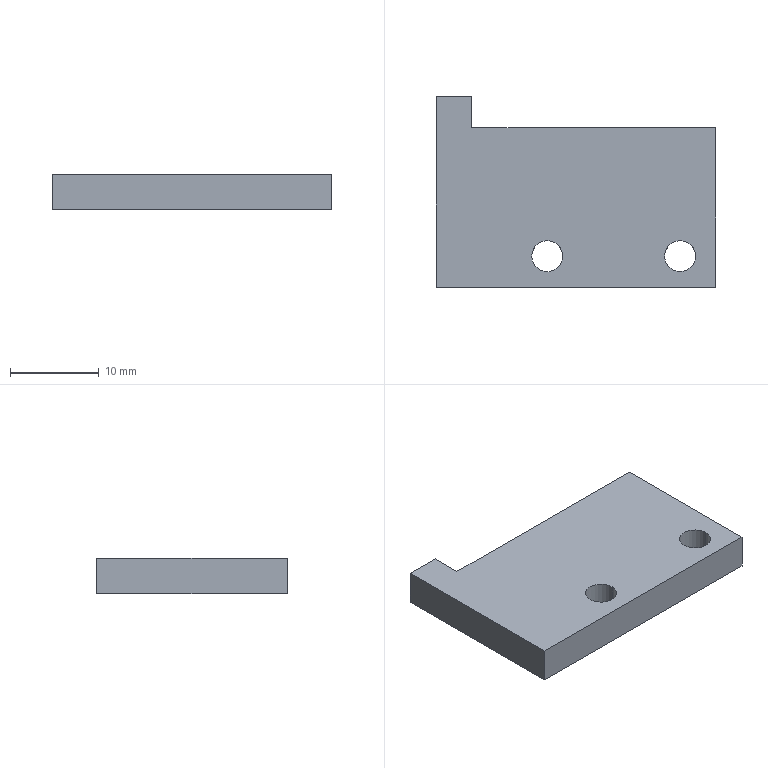Part | NX | 1 solid | 12 faces | box 31.5 x 21.5 x 4 mm | volume 2247 mm3 | plane 8 | cylinder 4 | commonest cylinder face diameters 3.5 x4
STEP:
#1=CARTESIAN_POINT('',(0.,-21.5,0.));
#2=VERTEX_POINT('',#1);
#3=CARTESIAN_POINT('',(0.,0.,0.));
#4=VERTEX_POINT('',#3);
#5=CARTESIAN_POINT('',(0.,0.,0.));
#6=DIRECTION('',(0.,1.,0.));
#7=VECTOR('',#6,1000.);
#8=LINE('',#5,#7);
#9=EDGE_CURVE('',#2,#4,#8,.T.);
#10=ORIENTED_EDGE('',*,*,#9,.T.);
#11=CARTESIAN_POINT('',(4.,0.,0.));
#12=VERTEX_POINT('',#11);
#13=CARTESIAN_POINT('',(0.,0.,0.));
#14=DIRECTION('',(1.,0.,0.));
#15=VECTOR('',#14,1000.);
#16=LINE('',#13,#15);
#17=EDGE_CURVE('',#4,#12,#16,.T.);
#18=ORIENTED_EDGE('',*,*,#17,.T.);
#19=CARTESIAN_POINT('',(4.,-3.5,0.));
#20=VERTEX_POINT('',#19);
#21=CARTESIAN_POINT('',(4.,0.,0.));
#22=DIRECTION('',(0.,-1.,0.));
#23=VECTOR('',#22,1000.);
#24=LINE('',#21,#23);
#25=EDGE_CURVE('',#12,#20,#24,.T.);
#26=ORIENTED_EDGE('',*,*,#25,.T.);
#27=CARTESIAN_POINT('',(31.5,-3.5,0.));
#28=VERTEX_POINT('',#27);
#29=CARTESIAN_POINT('',(0.,-3.5,0.));
#30=DIRECTION('',(1.,0.,0.));
#31=VECTOR('',#30,1000.);
#32=LINE('',#29,#31);
#33=EDGE_CURVE('',#20,#28,#32,.T.);
#34=ORIENTED_EDGE('',*,*,#33,.T.);
#35=CARTESIAN_POINT('',(31.5,-21.5,0.));
#36=VERTEX_POINT('',#35);
#37=CARTESIAN_POINT('',(31.5,0.,0.));
#38=DIRECTION('',(0.,1.,0.));
#39=VECTOR('',#38,1000.);
#40=LINE('',#37,#39);
#41=EDGE_CURVE('',#36,#28,#40,.T.);
#42=ORIENTED_EDGE('',*,*,#41,.F.);
#43=CARTESIAN_POINT('',(0.,-21.5,0.));
#44=DIRECTION('',(-1.,0.,0.));
#45=VECTOR('',#44,1000.);
#46=LINE('',#43,#45);
#47=EDGE_CURVE('',#36,#2,#46,.T.);
#48=ORIENTED_EDGE('',*,*,#47,.T.);
#49=EDGE_LOOP('',(#10,#18,#26,#34,#42,#48));
#50=FACE_BOUND('',#49,.T.);
#51=CARTESIAN_POINT('',(29.25,-18.,0.));
#52=VERTEX_POINT('',#51);
#53=CARTESIAN_POINT('',(25.75,-18.,0.));
#54=VERTEX_POINT('',#53);
#55=CARTESIAN_POINT('',(27.5,-18.,0.));
#56=DIRECTION('',(0.,0.,-1.));
#57=DIRECTION('',(-1.,0.,0.));
#58=AXIS2_PLACEMENT_3D('',#55,#56,#57);
#59=CIRCLE('',#58,1.75);
#60=EDGE_CURVE('',#52,#54,#59,.T.);
#61=ORIENTED_EDGE('',*,*,#60,.F.);
#62=CARTESIAN_POINT('',(27.5,-18.,0.));
#63=DIRECTION('',(0.,0.,-1.));
#64=DIRECTION('',(-1.,0.,0.));
#65=AXIS2_PLACEMENT_3D('',#62,#63,#64);
#66=CIRCLE('',#65,1.75);
#67=EDGE_CURVE('',#54,#52,#66,.T.);
#68=ORIENTED_EDGE('',*,*,#67,.F.);
#69=EDGE_LOOP('',(#61,#68));
#70=FACE_BOUND('',#69,.T.);
#71=CARTESIAN_POINT('',(14.25,-18.,0.));
#72=VERTEX_POINT('',#71);
#73=CARTESIAN_POINT('',(10.75,-18.,0.));
#74=VERTEX_POINT('',#73);
#75=CARTESIAN_POINT('',(12.5,-18.,0.));
#76=DIRECTION('',(0.,0.,-1.));
#77=DIRECTION('',(-1.,0.,0.));
#78=AXIS2_PLACEMENT_3D('',#75,#76,#77);
#79=CIRCLE('',#78,1.75);
#80=EDGE_CURVE('',#72,#74,#79,.T.);
#81=ORIENTED_EDGE('',*,*,#80,.F.);
#82=CARTESIAN_POINT('',(12.5,-18.,0.));
#83=DIRECTION('',(0.,0.,-1.));
#84=DIRECTION('',(-1.,0.,0.));
#85=AXIS2_PLACEMENT_3D('',#82,#83,#84);
#86=CIRCLE('',#85,1.75);
#87=EDGE_CURVE('',#74,#72,#86,.T.);
#88=ORIENTED_EDGE('',*,*,#87,.F.);
#89=EDGE_LOOP('',(#81,#88));
#90=FACE_BOUND('',#89,.T.);
#91=CARTESIAN_POINT('',(0.,0.,0.));
#92=DIRECTION('',(0.,0.,1.));
#93=DIRECTION('',(1.,0.,0.));
#94=AXIS2_PLACEMENT_3D('',#91,#92,#93);
#95=PLANE('',#94);
#96=ADVANCED_FACE('',(#50,#70,#90),#95,.F.);
#97=CARTESIAN_POINT('',(4.,0.,4.));
#98=VERTEX_POINT('',#97);
#99=CARTESIAN_POINT('',(4.,0.,0.));
#100=DIRECTION('',(0.,0.,1.));
#101=VECTOR('',#100,1000.);
#102=LINE('',#99,#101);
#103=EDGE_CURVE('',#12,#98,#102,.T.);
#104=ORIENTED_EDGE('',*,*,#103,.T.);
#105=CARTESIAN_POINT('',(4.,-3.5,4.));
#106=VERTEX_POINT('',#105);
#107=CARTESIAN_POINT('',(4.,0.,4.));
#108=DIRECTION('',(0.,1.,0.));
#109=VECTOR('',#108,1000.);
#110=LINE('',#107,#109);
#111=EDGE_CURVE('',#106,#98,#110,.T.);
#112=ORIENTED_EDGE('',*,*,#111,.F.);
#113=CARTESIAN_POINT('',(4.,-3.5,0.));
#114=DIRECTION('',(0.,0.,-1.));
#115=VECTOR('',#114,1000.);
#116=LINE('',#113,#115);
#117=EDGE_CURVE('',#106,#20,#116,.T.);
#118=ORIENTED_EDGE('',*,*,#117,.T.);
#119=ORIENTED_EDGE('',*,*,#25,.F.);
#120=EDGE_LOOP('',(#104,#112,#118,#119));
#121=FACE_BOUND('',#120,.T.);
#122=CARTESIAN_POINT('',(4.,0.,5.));
#123=DIRECTION('',(-1.,0.,0.));
#124=DIRECTION('',(0.,0.,1.));
#125=AXIS2_PLACEMENT_3D('',#122,#123,#124);
#126=PLANE('',#125);
#127=ADVANCED_FACE('',(#121),#126,.F.);
#128=CARTESIAN_POINT('',(0.,0.,4.));
#129=VERTEX_POINT('',#128);
#130=CARTESIAN_POINT('',(0.,0.,0.));
#131=DIRECTION('',(0.,0.,-1.));
#132=VECTOR('',#131,1000.);
#133=LINE('',#130,#132);
#134=EDGE_CURVE('',#129,#4,#133,.T.);
#135=ORIENTED_EDGE('',*,*,#134,.F.);
#136=CARTESIAN_POINT('',(0.,0.,4.));
#137=DIRECTION('',(-1.,0.,0.));
#138=VECTOR('',#137,1000.);
#139=LINE('',#136,#138);
#140=EDGE_CURVE('',#98,#129,#139,.T.);
#141=ORIENTED_EDGE('',*,*,#140,.F.);
#142=ORIENTED_EDGE('',*,*,#103,.F.);
#143=ORIENTED_EDGE('',*,*,#17,.F.);
#144=EDGE_LOOP('',(#135,#141,#142,#143));
#145=FACE_BOUND('',#144,.T.);
#146=CARTESIAN_POINT('',(32.,0.,0.));
#147=DIRECTION('',(0.,1.,0.));
#148=DIRECTION('',(1.,0.,0.));
#149=AXIS2_PLACEMENT_3D('',#146,#147,#148);
#150=PLANE('',#149);
#151=ADVANCED_FACE('',(#145),#150,.T.);
#152=CARTESIAN_POINT('',(0.,-21.5,4.));
#153=VERTEX_POINT('',#152);
#154=CARTESIAN_POINT('',(0.,-21.5,0.));
#155=DIRECTION('',(0.,0.,1.));
#156=VECTOR('',#155,1000.);
#157=LINE('',#154,#156);
#158=EDGE_CURVE('',#2,#153,#157,.T.);
#159=ORIENTED_EDGE('',*,*,#158,.T.);
#160=CARTESIAN_POINT('',(0.,0.,4.));
#161=DIRECTION('',(0.,-1.,0.));
#162=VECTOR('',#161,1000.);
#163=LINE('',#160,#162);
#164=EDGE_CURVE('',#129,#153,#163,.T.);
#165=ORIENTED_EDGE('',*,*,#164,.F.);
#166=ORIENTED_EDGE('',*,*,#134,.T.);
#167=ORIENTED_EDGE('',*,*,#9,.F.);
#168=EDGE_LOOP('',(#159,#165,#166,#167));
#169=FACE_BOUND('',#168,.T.);
#170=CARTESIAN_POINT('',(0.,0.,0.));
#171=DIRECTION('',(-1.,0.,0.));
#172=DIRECTION('',(0.,0.,1.));
#173=AXIS2_PLACEMENT_3D('',#170,#171,#172);
#174=PLANE('',#173);
#175=ADVANCED_FACE('',(#169),#174,.T.);
#176=CARTESIAN_POINT('',(31.5,-21.5,4.));
#177=VERTEX_POINT('',#176);
#178=CARTESIAN_POINT('',(0.,-21.5,4.));
#179=DIRECTION('',(1.,0.,0.));
#180=VECTOR('',#179,1000.);
#181=LINE('',#178,#180);
#182=EDGE_CURVE('',#153,#177,#181,.T.);
#183=ORIENTED_EDGE('',*,*,#182,.T.);
#184=CARTESIAN_POINT('',(31.5,-3.5,4.));
#185=VERTEX_POINT('',#184);
#186=CARTESIAN_POINT('',(31.5,0.,4.));
#187=DIRECTION('',(0.,-1.,0.));
#188=VECTOR('',#187,1000.);
#189=LINE('',#186,#188);
#190=EDGE_CURVE('',#185,#177,#189,.T.);
#191=ORIENTED_EDGE('',*,*,#190,.F.);
#192=CARTESIAN_POINT('',(0.,-3.5,4.));
#193=DIRECTION('',(1.,0.,0.));
#194=VECTOR('',#193,1000.);
#195=LINE('',#192,#194);
#196=EDGE_CURVE('',#106,#185,#195,.T.);
#197=ORIENTED_EDGE('',*,*,#196,.F.);
#198=ORIENTED_EDGE('',*,*,#111,.T.);
#199=ORIENTED_EDGE('',*,*,#140,.T.);
#200=ORIENTED_EDGE('',*,*,#164,.T.);
#201=EDGE_LOOP('',(#183,#191,#197,#198,#199,#200));
#202=FACE_BOUND('',#201,.T.);
#203=CARTESIAN_POINT('',(29.25,-18.,4.));
#204=VERTEX_POINT('',#203);
#205=CARTESIAN_POINT('',(25.75,-18.,4.));
#206=VERTEX_POINT('',#205);
#207=CARTESIAN_POINT('',(27.5,-18.,4.));
#208=DIRECTION('',(0.,0.,-1.));
#209=DIRECTION('',(-1.,0.,0.));
#210=AXIS2_PLACEMENT_3D('',#207,#208,#209);
#211=CIRCLE('',#210,1.75);
#212=EDGE_CURVE('',#204,#206,#211,.T.);
#213=ORIENTED_EDGE('',*,*,#212,.T.);
#214=CARTESIAN_POINT('',(27.5,-18.,4.));
#215=DIRECTION('',(0.,0.,-1.));
#216=DIRECTION('',(-1.,0.,0.));
#217=AXIS2_PLACEMENT_3D('',#214,#215,#216);
#218=CIRCLE('',#217,1.75);
#219=EDGE_CURVE('',#206,#204,#218,.T.);
#220=ORIENTED_EDGE('',*,*,#219,.T.);
#221=EDGE_LOOP('',(#213,#220));
#222=FACE_BOUND('',#221,.T.);
#223=CARTESIAN_POINT('',(10.75,-18.,4.));
#224=VERTEX_POINT('',#223);
#225=CARTESIAN_POINT('',(14.25,-18.,4.));
#226=VERTEX_POINT('',#225);
#227=CARTESIAN_POINT('',(12.5,-18.,4.));
#228=DIRECTION('',(0.,0.,-1.));
#229=DIRECTION('',(-1.,0.,0.));
#230=AXIS2_PLACEMENT_3D('',#227,#228,#229);
#231=CIRCLE('',#230,1.75);
#232=EDGE_CURVE('',#224,#226,#231,.T.);
#233=ORIENTED_EDGE('',*,*,#232,.T.);
#234=CARTESIAN_POINT('',(12.5,-18.,4.));
#235=DIRECTION('',(0.,0.,-1.));
#236=DIRECTION('',(-1.,0.,0.));
#237=AXIS2_PLACEMENT_3D('',#234,#235,#236);
#238=CIRCLE('',#237,1.75);
#239=EDGE_CURVE('',#226,#224,#238,.T.);
#240=ORIENTED_EDGE('',*,*,#239,.T.);
#241=EDGE_LOOP('',(#233,#240));
#242=FACE_BOUND('',#241,.T.);
#243=CARTESIAN_POINT('',(32.,-21.5,4.));
#244=DIRECTION('',(0.,0.,-1.));
#245=DIRECTION('',(0.,-1.,0.));
#246=AXIS2_PLACEMENT_3D('',#243,#244,#245);
#247=PLANE('',#246);
#248=ADVANCED_FACE('',(#202,#222,#242),#247,.F.);
#249=CARTESIAN_POINT('',(31.5,-3.5,0.));
#250=DIRECTION('',(0.,0.,1.));
#251=VECTOR('',#250,1000.);
#252=LINE('',#249,#251);
#253=EDGE_CURVE('',#28,#185,#252,.T.);
#254=ORIENTED_EDGE('',*,*,#253,.F.);
#255=ORIENTED_EDGE('',*,*,#33,.F.);
#256=ORIENTED_EDGE('',*,*,#117,.F.);
#257=ORIENTED_EDGE('',*,*,#196,.T.);
#258=EDGE_LOOP('',(#254,#255,#256,#257));
#259=FACE_BOUND('',#258,.T.);
#260=CARTESIAN_POINT('',(3.,-3.5,5.));
#261=DIRECTION('',(0.,-1.,0.));
#262=DIRECTION('',(0.,0.,-1.));
#263=AXIS2_PLACEMENT_3D('',#260,#261,#262);
#264=PLANE('',#263);
#265=ADVANCED_FACE('',(#259),#264,.F.);
#266=ORIENTED_EDGE('',*,*,#253,.T.);
#267=ORIENTED_EDGE('',*,*,#190,.T.);
#268=CARTESIAN_POINT('',(31.5,-21.5,0.));
#269=DIRECTION('',(0.,0.,1.));
#270=VECTOR('',#269,1000.);
#271=LINE('',#268,#270);
#272=EDGE_CURVE('',#36,#177,#271,.T.);
#273=ORIENTED_EDGE('',*,*,#272,.F.);
#274=ORIENTED_EDGE('',*,*,#41,.T.);
#275=EDGE_LOOP('',(#266,#267,#273,#274));
#276=FACE_BOUND('',#275,.T.);
#277=CARTESIAN_POINT('',(31.5,-22.5,0.));
#278=DIRECTION('',(1.,0.,0.));
#279=DIRECTION('',(0.,1.,0.));
#280=AXIS2_PLACEMENT_3D('',#277,#278,#279);
#281=PLANE('',#280);
#282=ADVANCED_FACE('',(#276),#281,.T.);
#283=ORIENTED_EDGE('',*,*,#158,.F.);
#284=ORIENTED_EDGE('',*,*,#47,.F.);
#285=ORIENTED_EDGE('',*,*,#272,.T.);
#286=ORIENTED_EDGE('',*,*,#182,.F.);
#287=EDGE_LOOP('',(#283,#284,#285,#286));
#288=FACE_BOUND('',#287,.T.);
#289=CARTESIAN_POINT('',(0.,-21.5,0.));
#290=DIRECTION('',(0.,-1.,0.));
#291=DIRECTION('',(0.,0.,-1.));
#292=AXIS2_PLACEMENT_3D('',#289,#290,#291);
#293=PLANE('',#292);
#294=ADVANCED_FACE('',(#288),#293,.T.);
#295=ORIENTED_EDGE('',*,*,#212,.F.);
#296=CARTESIAN_POINT('',(29.25,-18.,5.));
#297=DIRECTION('',(0.,0.,-1.));
#298=VECTOR('',#297,1000.);
#299=LINE('',#296,#298);
#300=EDGE_CURVE('',#52,#204,#299,.F.);
#301=ORIENTED_EDGE('',*,*,#300,.F.);
#302=ORIENTED_EDGE('',*,*,#60,.T.);
#303=CARTESIAN_POINT('',(25.75,-18.,5.));
#304=DIRECTION('',(0.,0.,-1.));
#305=VECTOR('',#304,1000.);
#306=LINE('',#303,#305);
#307=EDGE_CURVE('',#54,#206,#306,.F.);
#308=ORIENTED_EDGE('',*,*,#307,.T.);
#309=EDGE_LOOP('',(#295,#301,#302,#308));
#310=FACE_BOUND('',#309,.T.);
#311=CARTESIAN_POINT('',(27.5,-18.,5.));
#312=DIRECTION('',(0.,0.,-1.));
#313=DIRECTION('',(-1.,0.,0.));
#314=AXIS2_PLACEMENT_3D('',#311,#312,#313);
#315=CYLINDRICAL_SURFACE('',#314,1.75);
#316=ADVANCED_FACE('',(#310),#315,.F.);
#317=ORIENTED_EDGE('',*,*,#80,.T.);
#318=CARTESIAN_POINT('',(10.75,-18.,5.));
#319=DIRECTION('',(0.,0.,-1.));
#320=VECTOR('',#319,1000.);
#321=LINE('',#318,#320);
#322=EDGE_CURVE('',#74,#224,#321,.F.);
#323=ORIENTED_EDGE('',*,*,#322,.T.);
#324=ORIENTED_EDGE('',*,*,#239,.F.);
#325=CARTESIAN_POINT('',(14.25,-18.,5.));
#326=DIRECTION('',(0.,0.,-1.));
#327=VECTOR('',#326,1000.);
#328=LINE('',#325,#327);
#329=EDGE_CURVE('',#72,#226,#328,.F.);
#330=ORIENTED_EDGE('',*,*,#329,.F.);
#331=EDGE_LOOP('',(#317,#323,#324,#330));
#332=FACE_BOUND('',#331,.T.);
#333=CARTESIAN_POINT('',(12.5,-18.,5.));
#334=DIRECTION('',(0.,0.,-1.));
#335=DIRECTION('',(-1.,0.,0.));
#336=AXIS2_PLACEMENT_3D('',#333,#334,#335);
#337=CYLINDRICAL_SURFACE('',#336,1.75);
#338=ADVANCED_FACE('',(#332),#337,.F.);
#339=ORIENTED_EDGE('',*,*,#232,.F.);
#340=ORIENTED_EDGE('',*,*,#322,.F.);
#341=ORIENTED_EDGE('',*,*,#87,.T.);
#342=ORIENTED_EDGE('',*,*,#329,.T.);
#343=EDGE_LOOP('',(#339,#340,#341,#342));
#344=FACE_BOUND('',#343,.T.);
#345=CARTESIAN_POINT('',(12.5,-18.,5.));
#346=DIRECTION('',(0.,0.,-1.));
#347=DIRECTION('',(-1.,0.,0.));
#348=AXIS2_PLACEMENT_3D('',#345,#346,#347);
#349=CYLINDRICAL_SURFACE('',#348,1.75);
#350=ADVANCED_FACE('',(#344),#349,.F.);
#351=ORIENTED_EDGE('',*,*,#307,.F.);
#352=ORIENTED_EDGE('',*,*,#67,.T.);
#353=ORIENTED_EDGE('',*,*,#300,.T.);
#354=ORIENTED_EDGE('',*,*,#219,.F.);
#355=EDGE_LOOP('',(#351,#352,#353,#354));
#356=FACE_BOUND('',#355,.T.);
#357=CARTESIAN_POINT('',(27.5,-18.,5.));
#358=DIRECTION('',(0.,0.,-1.));
#359=DIRECTION('',(-1.,0.,0.));
#360=AXIS2_PLACEMENT_3D('',#357,#358,#359);
#361=CYLINDRICAL_SURFACE('',#360,1.75);
#362=ADVANCED_FACE('',(#356),#361,.F.);
#363=CLOSED_SHELL('',(#96,#127,#151,#175,#248,#265,#282,#294,#316,#338,#350,#362));
#364=MANIFOLD_SOLID_BREP('',#363);
#365=(LENGTH_UNIT()NAMED_UNIT(*)SI_UNIT(.MILLI.,.METRE.));
#366=UNCERTAINTY_MEASURE_WITH_UNIT(LENGTH_MEASURE(0.00001),#365,'','');
#367=(NAMED_UNIT(*)PLANE_ANGLE_UNIT()SI_UNIT($,.RADIAN.));
#368=(NAMED_UNIT(*)SI_UNIT($,.STERADIAN.)SOLID_ANGLE_UNIT());
#369=(GEOMETRIC_REPRESENTATION_CONTEXT(3)GLOBAL_UNCERTAINTY_ASSIGNED_CONTEXT((#366))GLOBAL_UNIT_ASSIGNED_CONTEXT((#365,#367,#368))REPRESENTATION_CONTEXT('',''));
#370=ADVANCED_BREP_SHAPE_REPRESENTATION('',(#364),#369);